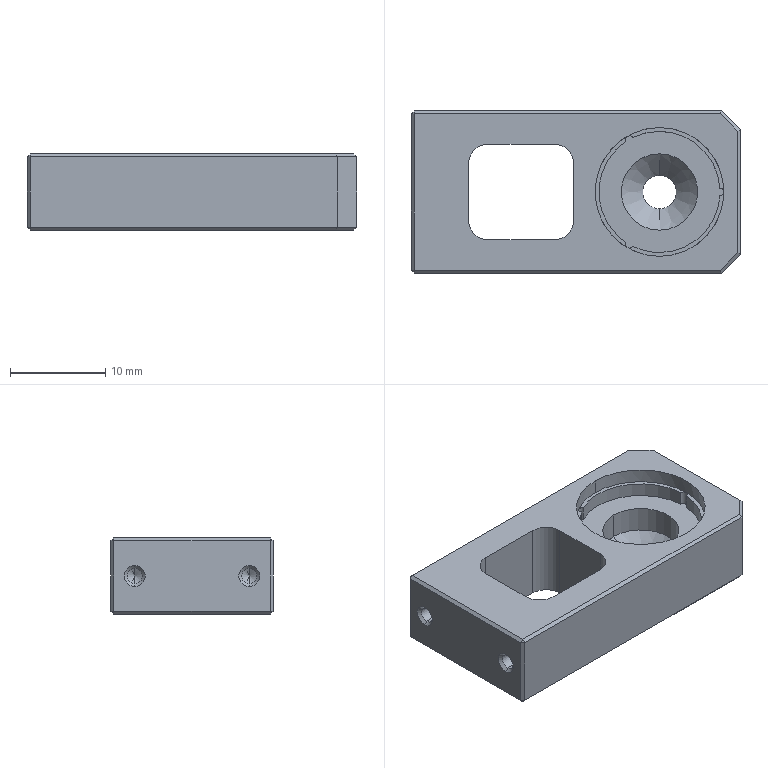Part | 1 solid | 66 faces | box 34.5 x 17 x 8 mm | volume 3172 mm3 | plane 34 | cylinder 22 | cone 10 | commonest cylinder face diameters 0.8 x6 1.6 x4 4 x4 12.7 x4 8 x2 13.5 x2